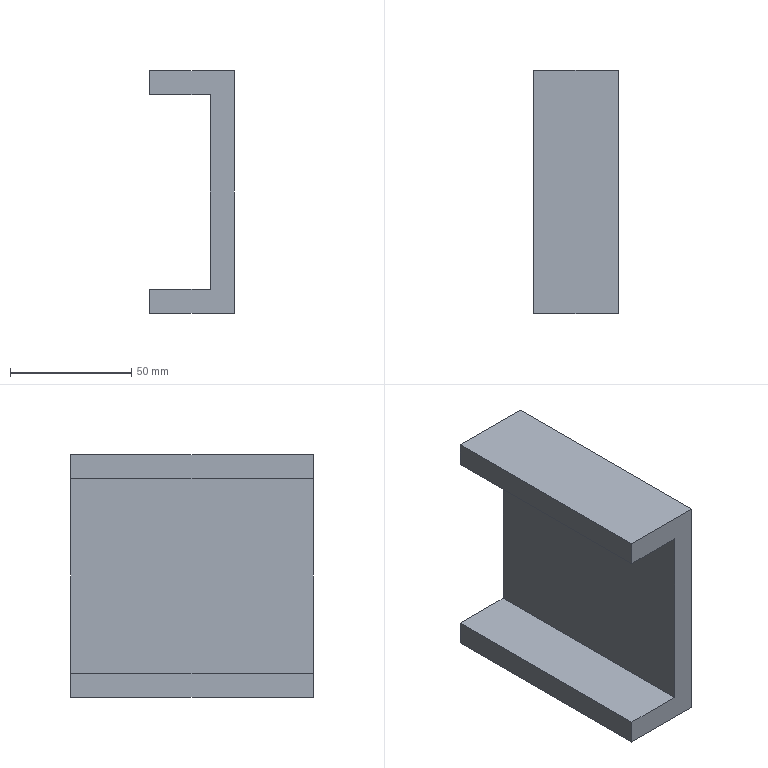Part | NX | 1 solid | 10 faces | box 35 x 100 x 100 mm | volume 150000 mm3 | plane 10
STEP:
#1=CARTESIAN_POINT('',(0.,-10.,-130.));
#2=VERTEX_POINT('',#1);
#3=CARTESIAN_POINT('',(0.,-110.,-130.));
#4=VERTEX_POINT('',#3);
#5=CARTESIAN_POINT('',(0.,0.,-130.));
#6=DIRECTION('',(0.,-1.,0.));
#7=VECTOR('',#6,1.);
#8=LINE('',#5,#7);
#9=EDGE_CURVE('',#2,#4,#8,.T.);
#10=ORIENTED_EDGE('',*,*,#9,.F.);
#11=CARTESIAN_POINT('',(-25.,-10.,-130.));
#12=VERTEX_POINT('',#11);
#13=CARTESIAN_POINT('',(13.,-10.,-130.));
#14=DIRECTION('',(-1.,0.,0.));
#15=VECTOR('',#14,1.);
#16=LINE('',#13,#15);
#17=EDGE_CURVE('',#2,#12,#16,.T.);
#18=ORIENTED_EDGE('',*,*,#17,.T.);
#19=CARTESIAN_POINT('',(-25.,-110.,-130.));
#20=VERTEX_POINT('',#19);
#21=CARTESIAN_POINT('',(-25.,0.,-130.));
#22=DIRECTION('',(0.,1.,0.));
#23=VECTOR('',#22,1.);
#24=LINE('',#21,#23);
#25=EDGE_CURVE('',#20,#12,#24,.T.);
#26=ORIENTED_EDGE('',*,*,#25,.F.);
#27=CARTESIAN_POINT('',(27.,-110.,-130.));
#28=DIRECTION('',(-1.,0.,0.));
#29=VECTOR('',#28,1.);
#30=LINE('',#27,#29);
#31=EDGE_CURVE('',#4,#20,#30,.T.);
#32=ORIENTED_EDGE('',*,*,#31,.F.);
#33=EDGE_LOOP('',(#10,#18,#26,#32));
#34=FACE_OUTER_BOUND('',#33,.T.);
#35=CARTESIAN_POINT('',(-8.725,-145.25,-130.));
#36=DIRECTION('',(0.,0.,-1.));
#37=DIRECTION('',(-1.,0.,0.));
#38=AXIS2_PLACEMENT_3D('',#35,#36,#37);
#39=PLANE('',#38);
#40=ADVANCED_FACE('',(#34),#39,.F.);
#41=CARTESIAN_POINT('',(-25.,-110.,-140.));
#42=VERTEX_POINT('',#41);
#43=CARTESIAN_POINT('',(-25.,-10.,-140.));
#44=VERTEX_POINT('',#43);
#45=CARTESIAN_POINT('',(-25.,422.25,-140.));
#46=DIRECTION('',(0.,1.,0.));
#47=VECTOR('',#46,1.);
#48=LINE('',#45,#47);
#49=EDGE_CURVE('',#42,#44,#48,.T.);
#50=ORIENTED_EDGE('',*,*,#49,.T.);
#51=CARTESIAN_POINT('',(10.,-10.,-140.));
#52=VERTEX_POINT('',#51);
#53=CARTESIAN_POINT('',(13.,-10.,-140.));
#54=DIRECTION('',(-1.,0.,0.));
#55=VECTOR('',#54,1.);
#56=LINE('',#53,#55);
#57=EDGE_CURVE('',#52,#44,#56,.T.);
#58=ORIENTED_EDGE('',*,*,#57,.F.);
#59=CARTESIAN_POINT('',(10.,-110.,-140.));
#60=VERTEX_POINT('',#59);
#61=CARTESIAN_POINT('',(10.,422.25,-140.));
#62=DIRECTION('',(0.,1.,0.));
#63=VECTOR('',#62,1.);
#64=LINE('',#61,#63);
#65=EDGE_CURVE('',#60,#52,#64,.T.);
#66=ORIENTED_EDGE('',*,*,#65,.F.);
#67=CARTESIAN_POINT('',(-1.5,-110.,-140.));
#68=DIRECTION('',(-1.,0.,0.));
#69=VECTOR('',#68,1.);
#70=LINE('',#67,#69);
#71=EDGE_CURVE('',#60,#42,#70,.T.);
#72=ORIENTED_EDGE('',*,*,#71,.T.);
#73=EDGE_LOOP('',(#50,#58,#66,#72));
#74=FACE_OUTER_BOUND('',#73,.T.);
#75=CARTESIAN_POINT('',(-1.5,422.25,-140.));
#76=DIRECTION('',(0.,0.,1.));
#77=DIRECTION('',(-1.,0.,0.));
#78=AXIS2_PLACEMENT_3D('',#75,#76,#77);
#79=PLANE('',#78);
#80=ADVANCED_FACE('',(#74),#79,.F.);
#81=CARTESIAN_POINT('',(10.,-10.,-40.));
#82=VERTEX_POINT('',#81);
#83=CARTESIAN_POINT('',(10.,-10.,-167.));
#84=DIRECTION('',(0.,0.,1.));
#85=VECTOR('',#84,1.);
#86=LINE('',#83,#85);
#87=EDGE_CURVE('',#52,#82,#86,.T.);
#88=ORIENTED_EDGE('',*,*,#87,.T.);
#89=CARTESIAN_POINT('',(10.,-110.,-40.));
#90=VERTEX_POINT('',#89);
#91=CARTESIAN_POINT('',(10.,422.25,-40.));
#92=DIRECTION('',(0.,-1.,0.));
#93=VECTOR('',#92,1.);
#94=LINE('',#91,#93);
#95=EDGE_CURVE('',#82,#90,#94,.T.);
#96=ORIENTED_EDGE('',*,*,#95,.T.);
#97=CARTESIAN_POINT('',(10.,-110.,-167.));
#98=DIRECTION('',(0.,0.,-1.));
#99=VECTOR('',#98,1.);
#100=LINE('',#97,#99);
#101=EDGE_CURVE('',#90,#60,#100,.T.);
#102=ORIENTED_EDGE('',*,*,#101,.T.);
#103=ORIENTED_EDGE('',*,*,#65,.T.);
#104=EDGE_LOOP('',(#88,#96,#102,#103));
#105=FACE_OUTER_BOUND('',#104,.T.);
#106=CARTESIAN_POINT('',(10.,0.,0.));
#107=DIRECTION('',(1.,0.,0.));
#108=DIRECTION('',(0.,0.,1.));
#109=AXIS2_PLACEMENT_3D('',#106,#107,#108);
#110=PLANE('',#109);
#111=ADVANCED_FACE('',(#105),#110,.T.);
#112=CARTESIAN_POINT('',(-25.,-110.,-167.));
#113=DIRECTION('',(0.,0.,-1.));
#114=VECTOR('',#113,1.);
#115=LINE('',#112,#114);
#116=EDGE_CURVE('',#20,#42,#115,.T.);
#117=ORIENTED_EDGE('',*,*,#116,.F.);
#118=ORIENTED_EDGE('',*,*,#25,.T.);
#119=CARTESIAN_POINT('',(-25.,-10.,-167.));
#120=DIRECTION('',(0.,0.,1.));
#121=VECTOR('',#120,1.);
#122=LINE('',#119,#121);
#123=EDGE_CURVE('',#44,#12,#122,.T.);
#124=ORIENTED_EDGE('',*,*,#123,.F.);
#125=ORIENTED_EDGE('',*,*,#49,.F.);
#126=EDGE_LOOP('',(#117,#118,#124,#125));
#127=FACE_OUTER_BOUND('',#126,.T.);
#128=CARTESIAN_POINT('',(-25.,0.,0.));
#129=DIRECTION('',(1.,0.,0.));
#130=DIRECTION('',(0.,0.,1.));
#131=AXIS2_PLACEMENT_3D('',#128,#129,#130);
#132=PLANE('',#131);
#133=ADVANCED_FACE('',(#127),#132,.F.);
#134=ORIENTED_EDGE('',*,*,#123,.T.);
#135=ORIENTED_EDGE('',*,*,#17,.F.);
#136=CARTESIAN_POINT('',(0.,-10.,-50.));
#137=VERTEX_POINT('',#136);
#138=CARTESIAN_POINT('',(0.,-10.,-167.));
#139=DIRECTION('',(0.,0.,1.));
#140=VECTOR('',#139,1.);
#141=LINE('',#138,#140);
#142=EDGE_CURVE('',#2,#137,#141,.T.);
#143=ORIENTED_EDGE('',*,*,#142,.T.);
#144=CARTESIAN_POINT('',(-25.,-10.,-50.));
#145=VERTEX_POINT('',#144);
#146=CARTESIAN_POINT('',(13.,-10.,-50.));
#147=DIRECTION('',(-1.,0.,0.));
#148=VECTOR('',#147,1.);
#149=LINE('',#146,#148);
#150=EDGE_CURVE('',#137,#145,#149,.T.);
#151=ORIENTED_EDGE('',*,*,#150,.T.);
#152=CARTESIAN_POINT('',(-25.,-10.,-40.));
#153=VERTEX_POINT('',#152);
#154=CARTESIAN_POINT('',(-25.,-10.,-167.));
#155=DIRECTION('',(0.,0.,1.));
#156=VECTOR('',#155,1.);
#157=LINE('',#154,#156);
#158=EDGE_CURVE('',#145,#153,#157,.T.);
#159=ORIENTED_EDGE('',*,*,#158,.T.);
#160=CARTESIAN_POINT('',(-15.95,-10.,-40.));
#161=DIRECTION('',(-1.,0.,0.));
#162=VECTOR('',#161,1.);
#163=LINE('',#160,#162);
#164=EDGE_CURVE('',#82,#153,#163,.T.);
#165=ORIENTED_EDGE('',*,*,#164,.F.);
#166=ORIENTED_EDGE('',*,*,#87,.F.);
#167=ORIENTED_EDGE('',*,*,#57,.T.);
#168=EDGE_LOOP('',(#134,#135,#143,#151,#159,#165,#166,#167));
#169=FACE_OUTER_BOUND('',#168,.T.);
#170=CARTESIAN_POINT('',(13.,-10.,-167.));
#171=DIRECTION('',(0.,-1.,0.));
#172=DIRECTION('',(0.,0.,1.));
#173=AXIS2_PLACEMENT_3D('',#170,#171,#172);
#174=PLANE('',#173);
#175=ADVANCED_FACE('',(#169),#174,.F.);
#176=ORIENTED_EDGE('',*,*,#101,.F.);
#177=CARTESIAN_POINT('',(-25.,-110.,-40.));
#178=VERTEX_POINT('',#177);
#179=CARTESIAN_POINT('',(27.,-110.,-40.));
#180=DIRECTION('',(-1.,0.,0.));
#181=VECTOR('',#180,1.);
#182=LINE('',#179,#181);
#183=EDGE_CURVE('',#90,#178,#182,.T.);
#184=ORIENTED_EDGE('',*,*,#183,.T.);
#185=CARTESIAN_POINT('',(-25.,-110.,-50.));
#186=VERTEX_POINT('',#185);
#187=CARTESIAN_POINT('',(-25.,-110.,-167.));
#188=DIRECTION('',(0.,0.,-1.));
#189=VECTOR('',#188,1.);
#190=LINE('',#187,#189);
#191=EDGE_CURVE('',#178,#186,#190,.T.);
#192=ORIENTED_EDGE('',*,*,#191,.T.);
#193=CARTESIAN_POINT('',(0.,-110.,-50.));
#194=VERTEX_POINT('',#193);
#195=CARTESIAN_POINT('',(27.,-110.,-50.));
#196=DIRECTION('',(-1.,0.,0.));
#197=VECTOR('',#196,1.);
#198=LINE('',#195,#197);
#199=EDGE_CURVE('',#194,#186,#198,.T.);
#200=ORIENTED_EDGE('',*,*,#199,.F.);
#201=CARTESIAN_POINT('',(0.,-110.,-167.));
#202=DIRECTION('',(0.,0.,-1.));
#203=VECTOR('',#202,1.);
#204=LINE('',#201,#203);
#205=EDGE_CURVE('',#194,#4,#204,.T.);
#206=ORIENTED_EDGE('',*,*,#205,.T.);
#207=ORIENTED_EDGE('',*,*,#31,.T.);
#208=ORIENTED_EDGE('',*,*,#116,.T.);
#209=ORIENTED_EDGE('',*,*,#71,.F.);
#210=EDGE_LOOP('',(#176,#184,#192,#200,#206,#207,#208,#209));
#211=FACE_OUTER_BOUND('',#210,.T.);
#212=CARTESIAN_POINT('',(27.,-110.,-167.));
#213=DIRECTION('',(0.,1.,0.));
#214=DIRECTION('',(0.,0.,-1.));
#215=AXIS2_PLACEMENT_3D('',#212,#213,#214);
#216=PLANE('',#215);
#217=ADVANCED_FACE('',(#211),#216,.F.);
#218=CARTESIAN_POINT('',(0.,0.,-50.));
#219=DIRECTION('',(0.,1.,0.));
#220=VECTOR('',#219,1.);
#221=LINE('',#218,#220);
#222=EDGE_CURVE('',#194,#137,#221,.T.);
#223=ORIENTED_EDGE('',*,*,#222,.T.);
#224=ORIENTED_EDGE('',*,*,#142,.F.);
#225=ORIENTED_EDGE('',*,*,#9,.T.);
#226=ORIENTED_EDGE('',*,*,#205,.F.);
#227=EDGE_LOOP('',(#223,#224,#225,#226));
#228=FACE_OUTER_BOUND('',#227,.T.);
#229=CARTESIAN_POINT('',(0.,0.,0.));
#230=DIRECTION('',(1.,0.,0.));
#231=DIRECTION('',(0.,0.,1.));
#232=AXIS2_PLACEMENT_3D('',#229,#230,#231);
#233=PLANE('',#232);
#234=ADVANCED_FACE('',(#228),#233,.F.);
#235=CARTESIAN_POINT('',(-25.,422.25,-40.));
#236=DIRECTION('',(0.,-1.,0.));
#237=VECTOR('',#236,1.);
#238=LINE('',#235,#237);
#239=EDGE_CURVE('',#153,#178,#238,.T.);
#240=ORIENTED_EDGE('',*,*,#239,.T.);
#241=ORIENTED_EDGE('',*,*,#183,.F.);
#242=ORIENTED_EDGE('',*,*,#95,.F.);
#243=ORIENTED_EDGE('',*,*,#164,.T.);
#244=EDGE_LOOP('',(#240,#241,#242,#243));
#245=FACE_OUTER_BOUND('',#244,.T.);
#246=CARTESIAN_POINT('',(-15.95,422.25,-40.));
#247=DIRECTION('',(0.,0.,-1.));
#248=DIRECTION('',(1.,0.,0.));
#249=AXIS2_PLACEMENT_3D('',#246,#247,#248);
#250=PLANE('',#249);
#251=ADVANCED_FACE('',(#245),#250,.F.);
#252=ORIENTED_EDGE('',*,*,#158,.F.);
#253=CARTESIAN_POINT('',(-25.,0.,-50.));
#254=DIRECTION('',(0.,-1.,0.));
#255=VECTOR('',#254,1.);
#256=LINE('',#253,#255);
#257=EDGE_CURVE('',#145,#186,#256,.T.);
#258=ORIENTED_EDGE('',*,*,#257,.T.);
#259=ORIENTED_EDGE('',*,*,#191,.F.);
#260=ORIENTED_EDGE('',*,*,#239,.F.);
#261=EDGE_LOOP('',(#252,#258,#259,#260));
#262=FACE_OUTER_BOUND('',#261,.T.);
#263=CARTESIAN_POINT('',(-25.,0.,0.));
#264=DIRECTION('',(1.,0.,0.));
#265=DIRECTION('',(0.,0.,1.));
#266=AXIS2_PLACEMENT_3D('',#263,#264,#265);
#267=PLANE('',#266);
#268=ADVANCED_FACE('',(#262),#267,.F.);
#269=ORIENTED_EDGE('',*,*,#222,.F.);
#270=ORIENTED_EDGE('',*,*,#199,.T.);
#271=ORIENTED_EDGE('',*,*,#257,.F.);
#272=ORIENTED_EDGE('',*,*,#150,.F.);
#273=EDGE_LOOP('',(#269,#270,#271,#272));
#274=FACE_OUTER_BOUND('',#273,.T.);
#275=CARTESIAN_POINT('',(-8.725,-145.25,-50.));
#276=DIRECTION('',(0.,0.,1.));
#277=DIRECTION('',(1.,0.,0.));
#278=AXIS2_PLACEMENT_3D('',#275,#276,#277);
#279=PLANE('',#278);
#280=ADVANCED_FACE('',(#274),#279,.F.);
#281=CLOSED_SHELL('',(#40,#80,#111,#133,#175,#217,#234,#251,#268,#280));
#282=MANIFOLD_SOLID_BREP('',#281);
#283=(LENGTH_UNIT()NAMED_UNIT(*)SI_UNIT(.MILLI.,.METRE.));
#284=UNCERTAINTY_MEASURE_WITH_UNIT(LENGTH_MEASURE(0.00002),#283,'','');
#285=(NAMED_UNIT(*)PLANE_ANGLE_UNIT()SI_UNIT($,.RADIAN.));
#286=PLANE_ANGLE_MEASURE_WITH_UNIT(PLANE_ANGLE_MEASURE(0.01745),#285);
#287=DIMENSIONAL_EXPONENTS(0.,0.,0.,0.,0.,0.,0.);
#288=(CONVERSION_BASED_UNIT('DEGREE',#286)NAMED_UNIT(#287)PLANE_ANGLE_UNIT());
#289=(NAMED_UNIT(*)SI_UNIT($,.STERADIAN.)SOLID_ANGLE_UNIT());
#290=(GEOMETRIC_REPRESENTATION_CONTEXT(3)GLOBAL_UNCERTAINTY_ASSIGNED_CONTEXT((#284))GLOBAL_UNIT_ASSIGNED_CONTEXT((#283,#288,#289))REPRESENTATION_CONTEXT('',''));
#291=ADVANCED_BREP_SHAPE_REPRESENTATION('',(#282),#290);